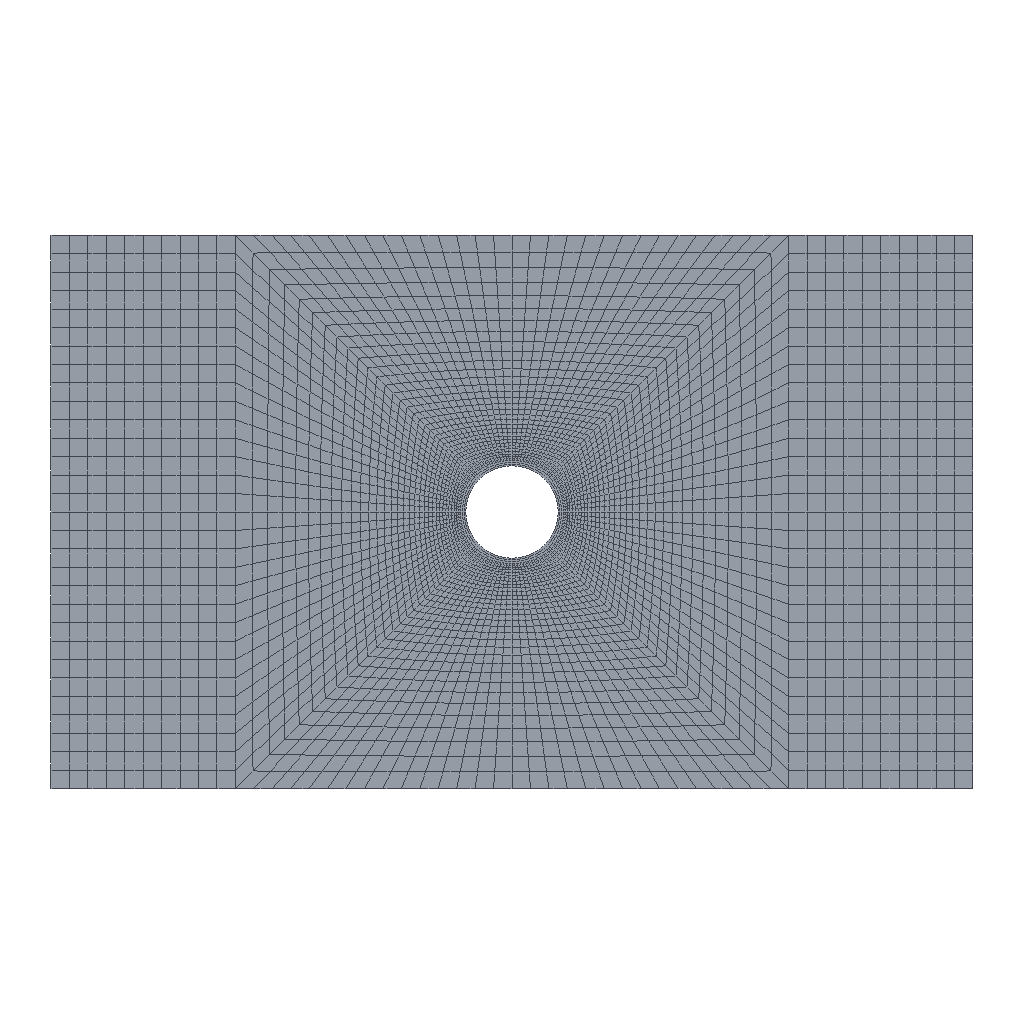Simulation study | abaqus
Set-up summary:
category,name,step,type,value,unit,region
solver,abaqus
solver,version,,,Abaqus/Standard 6.14-1
units,not stated in the deck,,not stated
analysis,deck,,static,static
load_step,Step-1,Step-1,static
load_step,requested,,,1
mesh,nodes,,,4940
mesh,elements,,,4800
element_type,S4R,,shell,4800
load,load commands in deck,,count,1
bc,support commands in deck,,count,8
material,MAT-T700,,in results
check,setup vs results,,match,"per instance, exact: element labels, types and connectivity; labels of the nodes the elements use; coordinates of those nodes at SINGLE_PRECISION in 1 of 1 instance(s)"
Abaqus input file, long lists of numbers shortened:
*Heading
** Job name: Job-Lam-1 Model name: Model-1
** Generated by: Abaqus/CAE 6.14-1
*Preprint, echo=NO, model=NO, history=NO, contact=NO
**
** PARTS
**
*Part, name=Lam-S
*Node
      1,          80.,          60.,           0.
      2,          80.,           0.,           0.
** (4938 more lines like these left out)
*Element, type=S4R
  1,   1,  13, 475,  88
  2,  13,  14, 476, 475
** (4798 more lines like these left out)
*Nset, nset=_PickedSet55, internal, generate
    1,  4940,     1
*Elset, elset=_PickedSet55, internal, generate
    1,  4800,     1
** Section: Sect-Lam
*Shell Section, elset=_PickedSet55, composite
0.15, 3, Mat-T700, 0., Layer-1
0.15, 3, Mat-T700, 45., Layer-2
0.15, 3, Mat-T700, -45., Layer-3
0.15, 3, Mat-T700, 90., Layer-4
*End Part
**
**
** ASSEMBLY
**
*Assembly, name=Assembly
**
*Instance, name=Lam-S-1, part=Lam-S
*End Instance
**
*Nset, nset=Nd-1, instance=Lam-S-1
 65,
*Nset, nset=_PickedSet38, internal, instance=Lam-S-1
   1,   2,   3,   4,   7,   8,   9,  10,  42,  43,  44,  45,  46,  47,  48,  49
  50,  80,  81,  82,  83,  84,  85,  86,  87,  88, 215, 216, 217, 218, 219, 220
** (5 more lines like these left out)
*Elset, elset=_PickedSet38, internal, instance=Lam-S-1
    1,   30,   31,   60,   61,   90,   91,  120,  121,  150,  151,  180,  181,  210,  211,  240
  241,  270,  271,  300, 1351, 1380, 1381, 1410, 1411, 1440, 1441, 1470, 1471, 1500, 1501, 1530
** (5 more lines like these left out)
*Nset, nset=_PickedSet39, internal, instance=Lam-S-1
  3,  4, 51, 52, 53, 54, 55, 56, 57, 58, 59, 60, 61, 62, 63, 64
 65, 66, 67, 68, 69, 70, 71, 72, 73, 74, 75, 76, 77, 78, 79
*Elset, elset=_PickedSet39, internal, instance=Lam-S-1, generate
 271,  300,    1
*Nset, nset=_PickedSet40, internal, instance=Lam-S-1
   9,  10, 224, 225, 226, 227, 228, 229, 230, 231, 232, 233, 234, 235, 236, 237
 238, 239, 240, 241, 242, 243, 244, 245, 246, 247, 248, 249, 250, 251, 252
*Elset, elset=_PickedSet40, internal, instance=Lam-S-1, generate
 1621,  1650,     1
*Surface, type=NODE, name=_PickedSet39_CNS_, internal
_PickedSet39, 1.
** Constraint: Constraint-1
*MPC
BEAM, _PickedSet39, Nd-1
*End Assembly
**
** MATERIALS
**
*Material, name=Mat-T700
*Elastic, type=LAMINA
114000.,8610.,  0.3,4160.,4160.,3000.
*Fail Stress
2688.,1458., 69.5, 236., 136.,   0.,   0.
**
** BOUNDARY CONDITIONS
**
** Name: BC-Left Type: Symmetry/Antisymmetry/Encastre
*Boundary
_PickedSet40, ENCASTRE
** Name: BC-Z Type: Displacement/Rotation
*Boundary
_PickedSet38, 3, 3
** ----------------------------------------------------------------
**
** STEP: Step-1
**
*Step, name=Step-1, nlgeom=NO
*Static
0.01, 1., 1e-05, 0.02
**
** BOUNDARY CONDITIONS
**
** Name: BC-X Type: Displacement/Rotation
*Boundary
Nd-1, 1, 1, -1.
Nd-1, 2, 2
Nd-1, 3, 3
Nd-1, 4, 4
Nd-1, 5, 5
Nd-1, 6, 6
**
** OUTPUT REQUESTS
**
*Restart, write, frequency=0
**
** FIELD OUTPUT: F-Output-1
**
*Output, field, time interval=0.02
*Node Output
U,
*Element Output, directions=YES
2, 5, 8, 11
CFAILURE, E, S
**
** HISTORY OUTPUT: H-Output-1
**
*Output, history, time interval=0.02
*Node Output, nset=Nd-1
RF1, U1
*End Step
Results summary:
result,step,Step-1,completed,increments=52 time=1.0/1.0
result,analysis,,,static
result,last_loadstep,,,1
result,primary field,,,"U, UR"